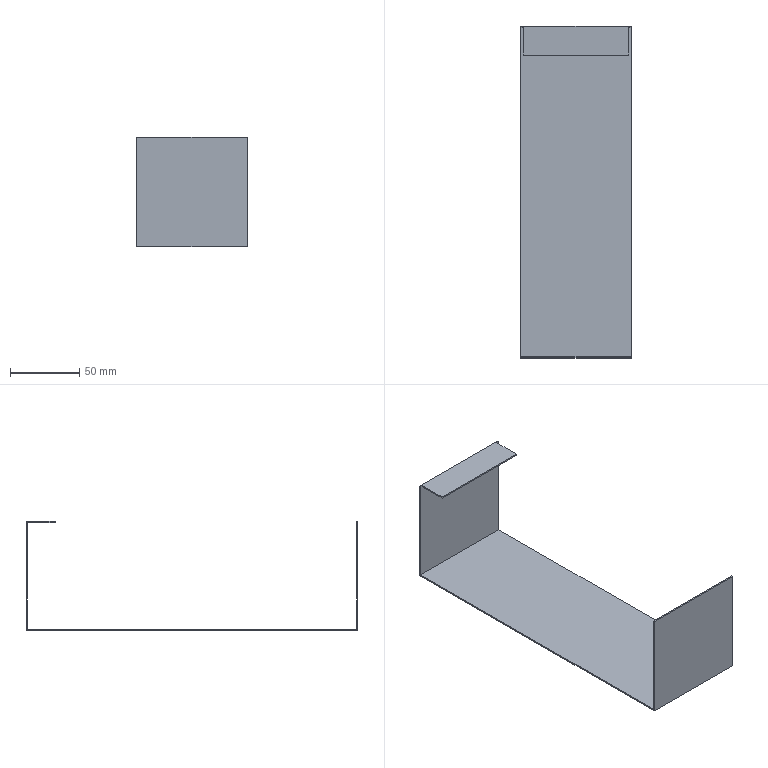Part | SolidWorks | features ICE 3, Extrusion 1 | 1 solid | 14 faces | box 80 x 240 x 79 mm | volume 33200 mm3 | plane 14
STEP:
#1=CARTESIAN_POINT('',(-40.,119.,79.));
#2=VERTEX_POINT('',#1);
#3=CARTESIAN_POINT('',(-38.,119.,79.));
#4=VERTEX_POINT('',#3);
#5=CARTESIAN_POINT('',(-40.,119.,79.));
#6=DIRECTION('',(1.,0.,0.));
#7=VECTOR('',#6,1000.);
#8=LINE('',#5,#7);
#9=EDGE_CURVE('',#2,#4,#8,.T.);
#10=ORIENTED_EDGE('',*,*,#9,.T.);
#11=CARTESIAN_POINT('',(-38.,99.,79.));
#12=VERTEX_POINT('',#11);
#13=CARTESIAN_POINT('',(-38.,121.236,79.));
#14=DIRECTION('',(0.,-1.,0.));
#15=VECTOR('',#14,1000.);
#16=LINE('',#13,#15);
#17=EDGE_CURVE('',#4,#12,#16,.T.);
#18=ORIENTED_EDGE('',*,*,#17,.T.);
#19=CARTESIAN_POINT('',(38.,99.,79.));
#20=VERTEX_POINT('',#19);
#21=CARTESIAN_POINT('',(-40.,99.,79.));
#22=DIRECTION('',(1.,0.,0.));
#23=VECTOR('',#22,1000.);
#24=LINE('',#21,#23);
#25=EDGE_CURVE('',#12,#20,#24,.T.);
#26=ORIENTED_EDGE('',*,*,#25,.T.);
#27=CARTESIAN_POINT('',(38.,119.,79.));
#28=VERTEX_POINT('',#27);
#29=CARTESIAN_POINT('',(38.,121.236,79.));
#30=DIRECTION('',(0.,-1.,0.));
#31=VECTOR('',#30,1000.);
#32=LINE('',#29,#31);
#33=EDGE_CURVE('',#28,#20,#32,.T.);
#34=ORIENTED_EDGE('',*,*,#33,.F.);
#35=CARTESIAN_POINT('',(40.,119.,79.));
#36=VERTEX_POINT('',#35);
#37=CARTESIAN_POINT('',(40.,119.,79.));
#38=DIRECTION('',(1.,0.,0.));
#39=VECTOR('',#38,1000.);
#40=LINE('',#37,#39);
#41=EDGE_CURVE('',#28,#36,#40,.T.);
#42=ORIENTED_EDGE('',*,*,#41,.T.);
#43=CARTESIAN_POINT('',(40.,120.,79.));
#44=VERTEX_POINT('',#43);
#45=CARTESIAN_POINT('',(40.,120.,79.));
#46=DIRECTION('',(0.,1.,0.));
#47=VECTOR('',#46,1000.);
#48=LINE('',#45,#47);
#49=EDGE_CURVE('',#36,#44,#48,.T.);
#50=ORIENTED_EDGE('',*,*,#49,.T.);
#51=CARTESIAN_POINT('',(-40.,120.,79.));
#52=VERTEX_POINT('',#51);
#53=CARTESIAN_POINT('',(-40.,120.,79.));
#54=DIRECTION('',(-1.,0.,0.));
#55=VECTOR('',#54,1000.);
#56=LINE('',#53,#55);
#57=EDGE_CURVE('',#44,#52,#56,.T.);
#58=ORIENTED_EDGE('',*,*,#57,.T.);
#59=CARTESIAN_POINT('',(-40.,120.,79.));
#60=DIRECTION('',(0.,-1.,0.));
#61=VECTOR('',#60,1000.);
#62=LINE('',#59,#61);
#63=EDGE_CURVE('',#52,#2,#62,.T.);
#64=ORIENTED_EDGE('',*,*,#63,.T.);
#65=EDGE_LOOP('',(#10,#18,#26,#34,#42,#50,#58,#64));
#66=FACE_OUTER_BOUND('',#65,.T.);
#67=CARTESIAN_POINT('',(0.,0.,79.));
#68=DIRECTION('',(0.,0.,1.));
#69=DIRECTION('',(1.,0.,0.));
#70=AXIS2_PLACEMENT_3D('',#67,#68,#69);
#71=PLANE('',#70);
#72=ADVANCED_FACE('',(#66),#71,.T.);
#73=ORIENTED_EDGE('',*,*,#25,.F.);
#74=CARTESIAN_POINT('',(-38.,99.,78.));
#75=VERTEX_POINT('',#74);
#76=CARTESIAN_POINT('',(-38.,99.,79.));
#77=DIRECTION('',(0.,0.,-1.));
#78=VECTOR('',#77,1000.);
#79=LINE('',#76,#78);
#80=EDGE_CURVE('',#12,#75,#79,.T.);
#81=ORIENTED_EDGE('',*,*,#80,.T.);
#82=CARTESIAN_POINT('',(38.,99.,78.));
#83=VERTEX_POINT('',#82);
#84=CARTESIAN_POINT('',(-40.,99.,78.));
#85=DIRECTION('',(1.,0.,0.));
#86=VECTOR('',#85,1000.);
#87=LINE('',#84,#86);
#88=EDGE_CURVE('',#75,#83,#87,.T.);
#89=ORIENTED_EDGE('',*,*,#88,.T.);
#90=CARTESIAN_POINT('',(38.,99.,79.));
#91=DIRECTION('',(0.,0.,1.));
#92=VECTOR('',#91,1000.);
#93=LINE('',#90,#92);
#94=EDGE_CURVE('',#83,#20,#93,.T.);
#95=ORIENTED_EDGE('',*,*,#94,.T.);
#96=EDGE_LOOP('',(#73,#81,#89,#95));
#97=FACE_OUTER_BOUND('',#96,.T.);
#98=CARTESIAN_POINT('',(-40.,99.,78.));
#99=DIRECTION('',(0.,-1.,0.));
#100=DIRECTION('',(0.,0.,-1.));
#101=AXIS2_PLACEMENT_3D('',#98,#99,#100);
#102=PLANE('',#101);
#103=ADVANCED_FACE('',(#97),#102,.T.);
#104=CARTESIAN_POINT('',(-38.,119.,78.));
#105=VERTEX_POINT('',#104);
#106=CARTESIAN_POINT('',(-38.,121.236,78.));
#107=DIRECTION('',(0.,-1.,0.));
#108=VECTOR('',#107,1000.);
#109=LINE('',#106,#108);
#110=EDGE_CURVE('',#105,#75,#109,.T.);
#111=ORIENTED_EDGE('',*,*,#110,.F.);
#112=CARTESIAN_POINT('',(38.,119.,78.));
#113=VERTEX_POINT('',#112);
#114=CARTESIAN_POINT('',(-40.,119.,78.));
#115=DIRECTION('',(-1.,0.,0.));
#116=VECTOR('',#115,1000.);
#117=LINE('',#114,#116);
#118=EDGE_CURVE('',#113,#105,#117,.T.);
#119=ORIENTED_EDGE('',*,*,#118,.F.);
#120=CARTESIAN_POINT('',(38.,121.236,78.));
#121=DIRECTION('',(0.,-1.,0.));
#122=VECTOR('',#121,1000.);
#123=LINE('',#120,#122);
#124=EDGE_CURVE('',#113,#83,#123,.T.);
#125=ORIENTED_EDGE('',*,*,#124,.T.);
#126=ORIENTED_EDGE('',*,*,#88,.F.);
#127=EDGE_LOOP('',(#111,#119,#125,#126));
#128=FACE_OUTER_BOUND('',#127,.T.);
#129=CARTESIAN_POINT('',(0.,0.,78.));
#130=DIRECTION('',(0.,0.,1.));
#131=DIRECTION('',(1.,0.,0.));
#132=AXIS2_PLACEMENT_3D('',#129,#130,#131);
#133=PLANE('',#132);
#134=ADVANCED_FACE('',(#128),#133,.F.);
#135=CARTESIAN_POINT('',(40.,119.,1.));
#136=VERTEX_POINT('',#135);
#137=CARTESIAN_POINT('',(40.,119.,79.));
#138=DIRECTION('',(0.,0.,-1.));
#139=VECTOR('',#138,1000.);
#140=LINE('',#137,#139);
#141=EDGE_CURVE('',#36,#136,#140,.T.);
#142=ORIENTED_EDGE('',*,*,#141,.F.);
#143=ORIENTED_EDGE('',*,*,#41,.F.);
#144=CARTESIAN_POINT('',(38.,119.,79.));
#145=DIRECTION('',(0.,0.,1.));
#146=VECTOR('',#145,1000.);
#147=LINE('',#144,#146);
#148=EDGE_CURVE('',#113,#28,#147,.T.);
#149=ORIENTED_EDGE('',*,*,#148,.F.);
#150=ORIENTED_EDGE('',*,*,#118,.T.);
#151=CARTESIAN_POINT('',(-38.,119.,79.));
#152=DIRECTION('',(0.,0.,-1.));
#153=VECTOR('',#152,1000.);
#154=LINE('',#151,#153);
#155=EDGE_CURVE('',#4,#105,#154,.T.);
#156=ORIENTED_EDGE('',*,*,#155,.F.);
#157=ORIENTED_EDGE('',*,*,#9,.F.);
#158=CARTESIAN_POINT('',(-40.,119.,1.));
#159=VERTEX_POINT('',#158);
#160=CARTESIAN_POINT('',(-40.,119.,79.));
#161=DIRECTION('',(0.,0.,-1.));
#162=VECTOR('',#161,1000.);
#163=LINE('',#160,#162);
#164=EDGE_CURVE('',#2,#159,#163,.T.);
#165=ORIENTED_EDGE('',*,*,#164,.T.);
#166=CARTESIAN_POINT('',(-40.,119.,1.));
#167=DIRECTION('',(1.,0.,0.));
#168=VECTOR('',#167,1000.);
#169=LINE('',#166,#168);
#170=EDGE_CURVE('',#159,#136,#169,.T.);
#171=ORIENTED_EDGE('',*,*,#170,.T.);
#172=EDGE_LOOP('',(#142,#143,#149,#150,#156,#157,#165,#171));
#173=FACE_OUTER_BOUND('',#172,.T.);
#174=CARTESIAN_POINT('',(-40.,119.,79.));
#175=DIRECTION('',(0.,1.,0.));
#176=DIRECTION('',(0.,0.,1.));
#177=AXIS2_PLACEMENT_3D('',#174,#175,#176);
#178=PLANE('',#177);
#179=ADVANCED_FACE('',(#173),#178,.F.);
#180=CARTESIAN_POINT('',(-40.,-119.,1.));
#181=VERTEX_POINT('',#180);
#182=CARTESIAN_POINT('',(-40.,120.,1.));
#183=DIRECTION('',(0.,-1.,0.));
#184=VECTOR('',#183,1000.);
#185=LINE('',#182,#184);
#186=EDGE_CURVE('',#159,#181,#185,.T.);
#187=ORIENTED_EDGE('',*,*,#186,.T.);
#188=CARTESIAN_POINT('',(40.,-119.,1.));
#189=VERTEX_POINT('',#188);
#190=CARTESIAN_POINT('',(-40.,-119.,1.));
#191=DIRECTION('',(-1.,0.,0.));
#192=VECTOR('',#191,1000.);
#193=LINE('',#190,#192);
#194=EDGE_CURVE('',#189,#181,#193,.T.);
#195=ORIENTED_EDGE('',*,*,#194,.F.);
#196=CARTESIAN_POINT('',(40.,120.,1.));
#197=DIRECTION('',(0.,1.,0.));
#198=VECTOR('',#197,1000.);
#199=LINE('',#196,#198);
#200=EDGE_CURVE('',#189,#136,#199,.T.);
#201=ORIENTED_EDGE('',*,*,#200,.T.);
#202=ORIENTED_EDGE('',*,*,#170,.F.);
#203=EDGE_LOOP('',(#187,#195,#201,#202));
#204=FACE_OUTER_BOUND('',#203,.T.);
#205=CARTESIAN_POINT('',(0.,0.,1.));
#206=DIRECTION('',(0.,0.,1.));
#207=DIRECTION('',(1.,0.,0.));
#208=AXIS2_PLACEMENT_3D('',#205,#206,#207);
#209=PLANE('',#208);
#210=ADVANCED_FACE('',(#204),#209,.T.);
#211=ORIENTED_EDGE('',*,*,#49,.F.);
#212=ORIENTED_EDGE('',*,*,#141,.T.);
#213=ORIENTED_EDGE('',*,*,#200,.F.);
#214=CARTESIAN_POINT('',(40.,-119.,79.));
#215=VERTEX_POINT('',#214);
#216=CARTESIAN_POINT('',(40.,-119.,79.));
#217=DIRECTION('',(0.,0.,-1.));
#218=VECTOR('',#217,1000.);
#219=LINE('',#216,#218);
#220=EDGE_CURVE('',#215,#189,#219,.T.);
#221=ORIENTED_EDGE('',*,*,#220,.F.);
#222=CARTESIAN_POINT('',(40.,-120.,79.));
#223=VERTEX_POINT('',#222);
#224=CARTESIAN_POINT('',(40.,-120.,79.));
#225=DIRECTION('',(0.,1.,0.));
#226=VECTOR('',#225,1000.);
#227=LINE('',#224,#226);
#228=EDGE_CURVE('',#223,#215,#227,.T.);
#229=ORIENTED_EDGE('',*,*,#228,.F.);
#230=CARTESIAN_POINT('',(40.,-120.,0.));
#231=VERTEX_POINT('',#230);
#232=CARTESIAN_POINT('',(40.,-120.,1.));
#233=DIRECTION('',(0.,0.,-1.));
#234=VECTOR('',#233,1000.);
#235=LINE('',#232,#234);
#236=EDGE_CURVE('',#223,#231,#235,.T.);
#237=ORIENTED_EDGE('',*,*,#236,.T.);
#238=CARTESIAN_POINT('',(40.,120.,0.));
#239=VERTEX_POINT('',#238);
#240=CARTESIAN_POINT('',(40.,120.,0.));
#241=DIRECTION('',(0.,1.,0.));
#242=VECTOR('',#241,1000.);
#243=LINE('',#240,#242);
#244=EDGE_CURVE('',#231,#239,#243,.T.);
#245=ORIENTED_EDGE('',*,*,#244,.T.);
#246=CARTESIAN_POINT('',(40.,120.,1.));
#247=DIRECTION('',(0.,0.,-1.));
#248=VECTOR('',#247,1000.);
#249=LINE('',#246,#248);
#250=EDGE_CURVE('',#44,#239,#249,.T.);
#251=ORIENTED_EDGE('',*,*,#250,.F.);
#252=EDGE_LOOP('',(#211,#212,#213,#221,#229,#237,#245,#251));
#253=FACE_OUTER_BOUND('',#252,.T.);
#254=CARTESIAN_POINT('',(40.,120.,1.));
#255=DIRECTION('',(-1.,0.,0.));
#256=DIRECTION('',(0.,-1.,0.));
#257=AXIS2_PLACEMENT_3D('',#254,#255,#256);
#258=PLANE('',#257);
#259=ADVANCED_FACE('',(#253),#258,.F.);
#260=CARTESIAN_POINT('',(-40.,120.,0.));
#261=VERTEX_POINT('',#260);
#262=CARTESIAN_POINT('',(-40.,120.,0.));
#263=DIRECTION('',(-1.,0.,0.));
#264=VECTOR('',#263,1000.);
#265=LINE('',#262,#264);
#266=EDGE_CURVE('',#239,#261,#265,.T.);
#267=ORIENTED_EDGE('',*,*,#266,.T.);
#268=CARTESIAN_POINT('',(-40.,120.,1.));
#269=DIRECTION('',(0.,0.,-1.));
#270=VECTOR('',#269,1000.);
#271=LINE('',#268,#270);
#272=EDGE_CURVE('',#52,#261,#271,.T.);
#273=ORIENTED_EDGE('',*,*,#272,.F.);
#274=ORIENTED_EDGE('',*,*,#57,.F.);
#275=ORIENTED_EDGE('',*,*,#250,.T.);
#276=EDGE_LOOP('',(#267,#273,#274,#275));
#277=FACE_OUTER_BOUND('',#276,.T.);
#278=CARTESIAN_POINT('',(-40.,120.,1.));
#279=DIRECTION('',(0.,-1.,0.));
#280=DIRECTION('',(0.,0.,-1.));
#281=AXIS2_PLACEMENT_3D('',#278,#279,#280);
#282=PLANE('',#281);
#283=ADVANCED_FACE('',(#277),#282,.F.);
#284=ORIENTED_EDGE('',*,*,#164,.F.);
#285=ORIENTED_EDGE('',*,*,#63,.F.);
#286=ORIENTED_EDGE('',*,*,#272,.T.);
#287=CARTESIAN_POINT('',(-40.,-120.,0.));
#288=VERTEX_POINT('',#287);
#289=CARTESIAN_POINT('',(-40.,120.,0.));
#290=DIRECTION('',(0.,-1.,0.));
#291=VECTOR('',#290,1000.);
#292=LINE('',#289,#291);
#293=EDGE_CURVE('',#261,#288,#292,.T.);
#294=ORIENTED_EDGE('',*,*,#293,.T.);
#295=CARTESIAN_POINT('',(-40.,-120.,79.));
#296=VERTEX_POINT('',#295);
#297=CARTESIAN_POINT('',(-40.,-120.,1.));
#298=DIRECTION('',(0.,0.,-1.));
#299=VECTOR('',#298,1000.);
#300=LINE('',#297,#299);
#301=EDGE_CURVE('',#296,#288,#300,.T.);
#302=ORIENTED_EDGE('',*,*,#301,.F.);
#303=CARTESIAN_POINT('',(-40.,-119.,79.));
#304=VERTEX_POINT('',#303);
#305=CARTESIAN_POINT('',(-40.,-120.,79.));
#306=DIRECTION('',(0.,-1.,0.));
#307=VECTOR('',#306,1000.);
#308=LINE('',#305,#307);
#309=EDGE_CURVE('',#304,#296,#308,.T.);
#310=ORIENTED_EDGE('',*,*,#309,.F.);
#311=CARTESIAN_POINT('',(-40.,-119.,79.));
#312=DIRECTION('',(0.,0.,-1.));
#313=VECTOR('',#312,1000.);
#314=LINE('',#311,#313);
#315=EDGE_CURVE('',#304,#181,#314,.T.);
#316=ORIENTED_EDGE('',*,*,#315,.T.);
#317=ORIENTED_EDGE('',*,*,#186,.F.);
#318=EDGE_LOOP('',(#284,#285,#286,#294,#302,#310,#316,#317));
#319=FACE_OUTER_BOUND('',#318,.T.);
#320=CARTESIAN_POINT('',(-40.,120.,1.));
#321=DIRECTION('',(1.,0.,0.));
#322=DIRECTION('',(0.,1.,0.));
#323=AXIS2_PLACEMENT_3D('',#320,#321,#322);
#324=PLANE('',#323);
#325=ADVANCED_FACE('',(#319),#324,.F.);
#326=CARTESIAN_POINT('',(-40.,-120.,0.));
#327=DIRECTION('',(1.,0.,0.));
#328=VECTOR('',#327,1000.);
#329=LINE('',#326,#328);
#330=EDGE_CURVE('',#288,#231,#329,.T.);
#331=ORIENTED_EDGE('',*,*,#330,.T.);
#332=ORIENTED_EDGE('',*,*,#236,.F.);
#333=CARTESIAN_POINT('',(-40.,-120.,79.));
#334=DIRECTION('',(1.,0.,0.));
#335=VECTOR('',#334,1000.);
#336=LINE('',#333,#335);
#337=EDGE_CURVE('',#296,#223,#336,.T.);
#338=ORIENTED_EDGE('',*,*,#337,.F.);
#339=ORIENTED_EDGE('',*,*,#301,.T.);
#340=EDGE_LOOP('',(#331,#332,#338,#339));
#341=FACE_OUTER_BOUND('',#340,.T.);
#342=CARTESIAN_POINT('',(-40.,-120.,1.));
#343=DIRECTION('',(0.,1.,0.));
#344=DIRECTION('',(0.,0.,1.));
#345=AXIS2_PLACEMENT_3D('',#342,#343,#344);
#346=PLANE('',#345);
#347=ADVANCED_FACE('',(#341),#346,.F.);
#348=ORIENTED_EDGE('',*,*,#244,.F.);
#349=ORIENTED_EDGE('',*,*,#330,.F.);
#350=ORIENTED_EDGE('',*,*,#293,.F.);
#351=ORIENTED_EDGE('',*,*,#266,.F.);
#352=EDGE_LOOP('',(#348,#349,#350,#351));
#353=FACE_OUTER_BOUND('',#352,.T.);
#354=CARTESIAN_POINT('',(0.,0.,0.));
#355=DIRECTION('',(0.,0.,1.));
#356=DIRECTION('',(1.,0.,0.));
#357=AXIS2_PLACEMENT_3D('',#354,#355,#356);
#358=PLANE('',#357);
#359=ADVANCED_FACE('',(#353),#358,.F.);
#360=ORIENTED_EDGE('',*,*,#194,.T.);
#361=ORIENTED_EDGE('',*,*,#315,.F.);
#362=CARTESIAN_POINT('',(-40.,-119.,79.));
#363=DIRECTION('',(-1.,0.,0.));
#364=VECTOR('',#363,1000.);
#365=LINE('',#362,#364);
#366=EDGE_CURVE('',#215,#304,#365,.T.);
#367=ORIENTED_EDGE('',*,*,#366,.F.);
#368=ORIENTED_EDGE('',*,*,#220,.T.);
#369=EDGE_LOOP('',(#360,#361,#367,#368));
#370=FACE_OUTER_BOUND('',#369,.T.);
#371=CARTESIAN_POINT('',(-40.,-119.,79.));
#372=DIRECTION('',(0.,-1.,0.));
#373=DIRECTION('',(0.,0.,-1.));
#374=AXIS2_PLACEMENT_3D('',#371,#372,#373);
#375=PLANE('',#374);
#376=ADVANCED_FACE('',(#370),#375,.F.);
#377=ORIENTED_EDGE('',*,*,#309,.T.);
#378=ORIENTED_EDGE('',*,*,#337,.T.);
#379=ORIENTED_EDGE('',*,*,#228,.T.);
#380=ORIENTED_EDGE('',*,*,#366,.T.);
#381=EDGE_LOOP('',(#377,#378,#379,#380));
#382=FACE_OUTER_BOUND('',#381,.T.);
#383=CARTESIAN_POINT('',(0.,0.,79.));
#384=DIRECTION('',(0.,0.,-1.));
#385=DIRECTION('',(-1.,0.,0.));
#386=AXIS2_PLACEMENT_3D('',#383,#384,#385);
#387=PLANE('',#386);
#388=ADVANCED_FACE('',(#382),#387,.F.);
#389=ORIENTED_EDGE('',*,*,#148,.T.);
#390=ORIENTED_EDGE('',*,*,#33,.T.);
#391=ORIENTED_EDGE('',*,*,#94,.F.);
#392=ORIENTED_EDGE('',*,*,#124,.F.);
#393=EDGE_LOOP('',(#389,#390,#391,#392));
#394=FACE_OUTER_BOUND('',#393,.T.);
#395=CARTESIAN_POINT('',(38.,121.236,79.));
#396=DIRECTION('',(1.,0.,0.));
#397=DIRECTION('',(0.,0.,-1.));
#398=AXIS2_PLACEMENT_3D('',#395,#396,#397);
#399=PLANE('',#398);
#400=ADVANCED_FACE('',(#394),#399,.T.);
#401=ORIENTED_EDGE('',*,*,#155,.T.);
#402=ORIENTED_EDGE('',*,*,#110,.T.);
#403=ORIENTED_EDGE('',*,*,#80,.F.);
#404=ORIENTED_EDGE('',*,*,#17,.F.);
#405=EDGE_LOOP('',(#401,#402,#403,#404));
#406=FACE_OUTER_BOUND('',#405,.T.);
#407=CARTESIAN_POINT('',(-38.,121.236,79.));
#408=DIRECTION('',(-1.,0.,0.));
#409=DIRECTION('',(0.,0.,1.));
#410=AXIS2_PLACEMENT_3D('',#407,#408,#409);
#411=PLANE('',#410);
#412=ADVANCED_FACE('',(#406),#411,.T.);
#413=CLOSED_SHELL('',(#72,#103,#134,#179,#210,#259,#283,#325,#347,#359,#376,#388,#400,#412));
#414=MANIFOLD_SOLID_BREP('',#413);
#415=CARTESIAN_POINT('',(0.,0.,0.));
#416=DIRECTION('',(0.,0.,1.));
#417=DIRECTION('',(1.,0.,0.));
#418=AXIS2_PLACEMENT_3D('',#415,#416,#417);
#419=(LENGTH_UNIT()NAMED_UNIT(*)SI_UNIT(.MILLI.,.METRE.));
#420=UNCERTAINTY_MEASURE_WITH_UNIT(LENGTH_MEASURE(0.00001),#419,'','');
#421=(NAMED_UNIT(*)PLANE_ANGLE_UNIT()SI_UNIT($,.RADIAN.));
#422=(NAMED_UNIT(*)SI_UNIT($,.STERADIAN.)SOLID_ANGLE_UNIT());
#423=(GEOMETRIC_REPRESENTATION_CONTEXT(3)GLOBAL_UNCERTAINTY_ASSIGNED_CONTEXT((#420))GLOBAL_UNIT_ASSIGNED_CONTEXT((#419,#421,#422))REPRESENTATION_CONTEXT('',''));
#424=ADVANCED_BREP_SHAPE_REPRESENTATION('',(#414,#418),#423);